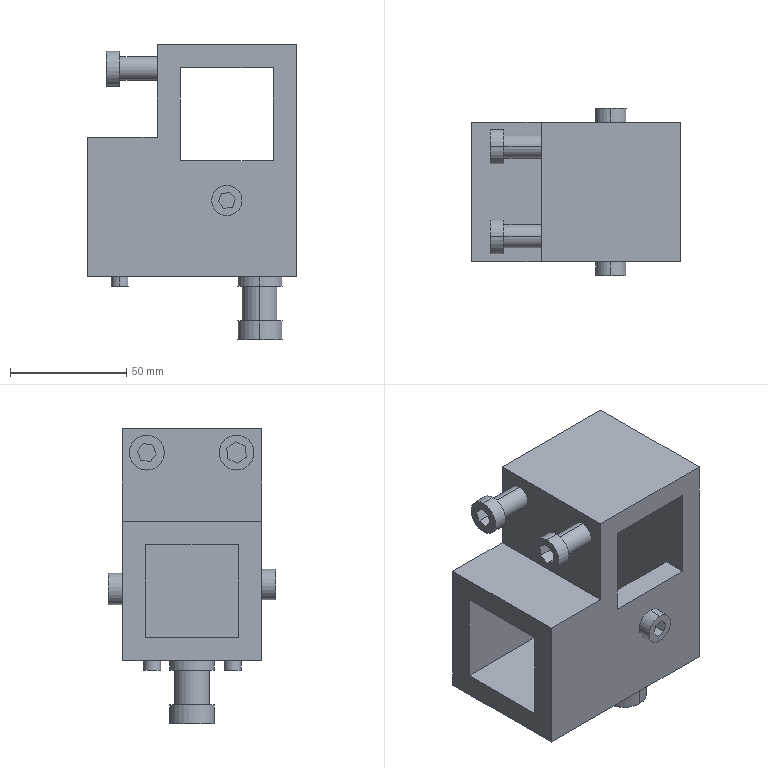Part | SolidWorks | features ICE 12, Extrusion 1 | 1 solid | 96 faces | box 90 x 72 x 127 mm | volume 255195 mm3 | plane 70 | cylinder 26 | commonest cylinder face diameters 6 x4 10 x4 19.302 x4 7.362 x2 7.454 x2 13.083 x2